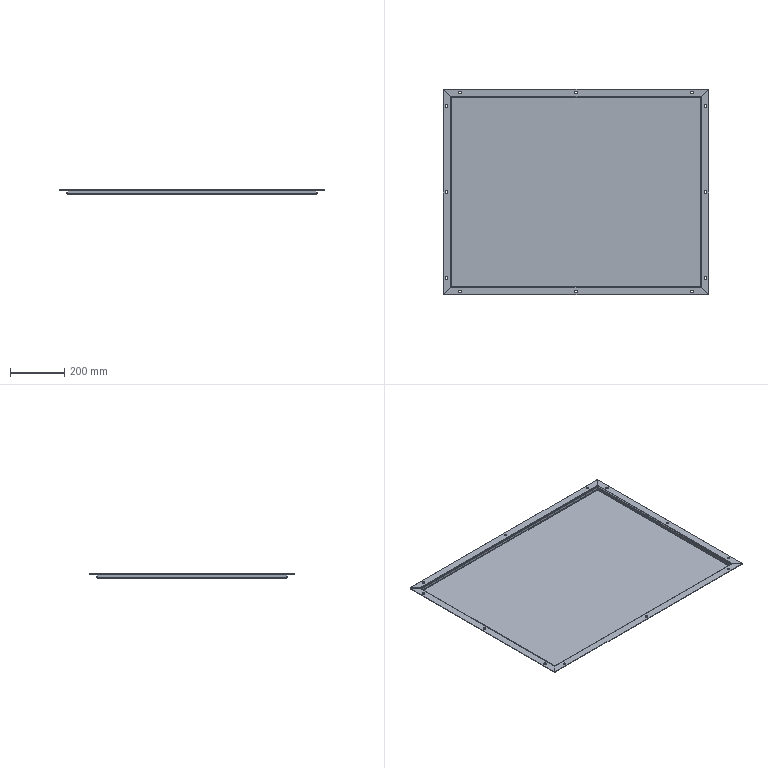Part | STEP file | 750078271 | 1 solid | 102 faces | box 979 x 758 x 17 mm | volume 1562109 mm3 | plane 54 | cylinder 48 | commonest cylinder face diameters 10 x32 4 x8 8 x8